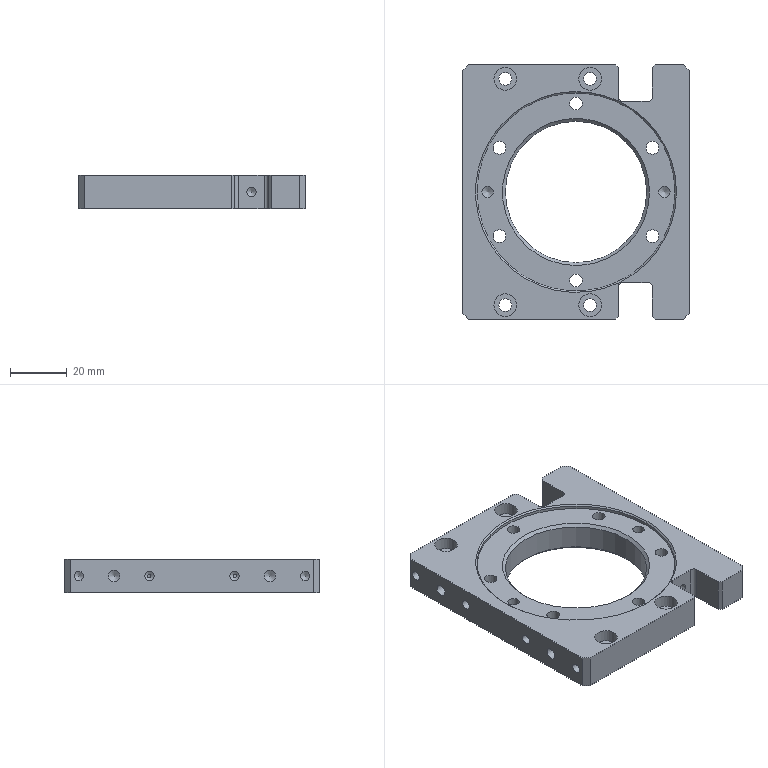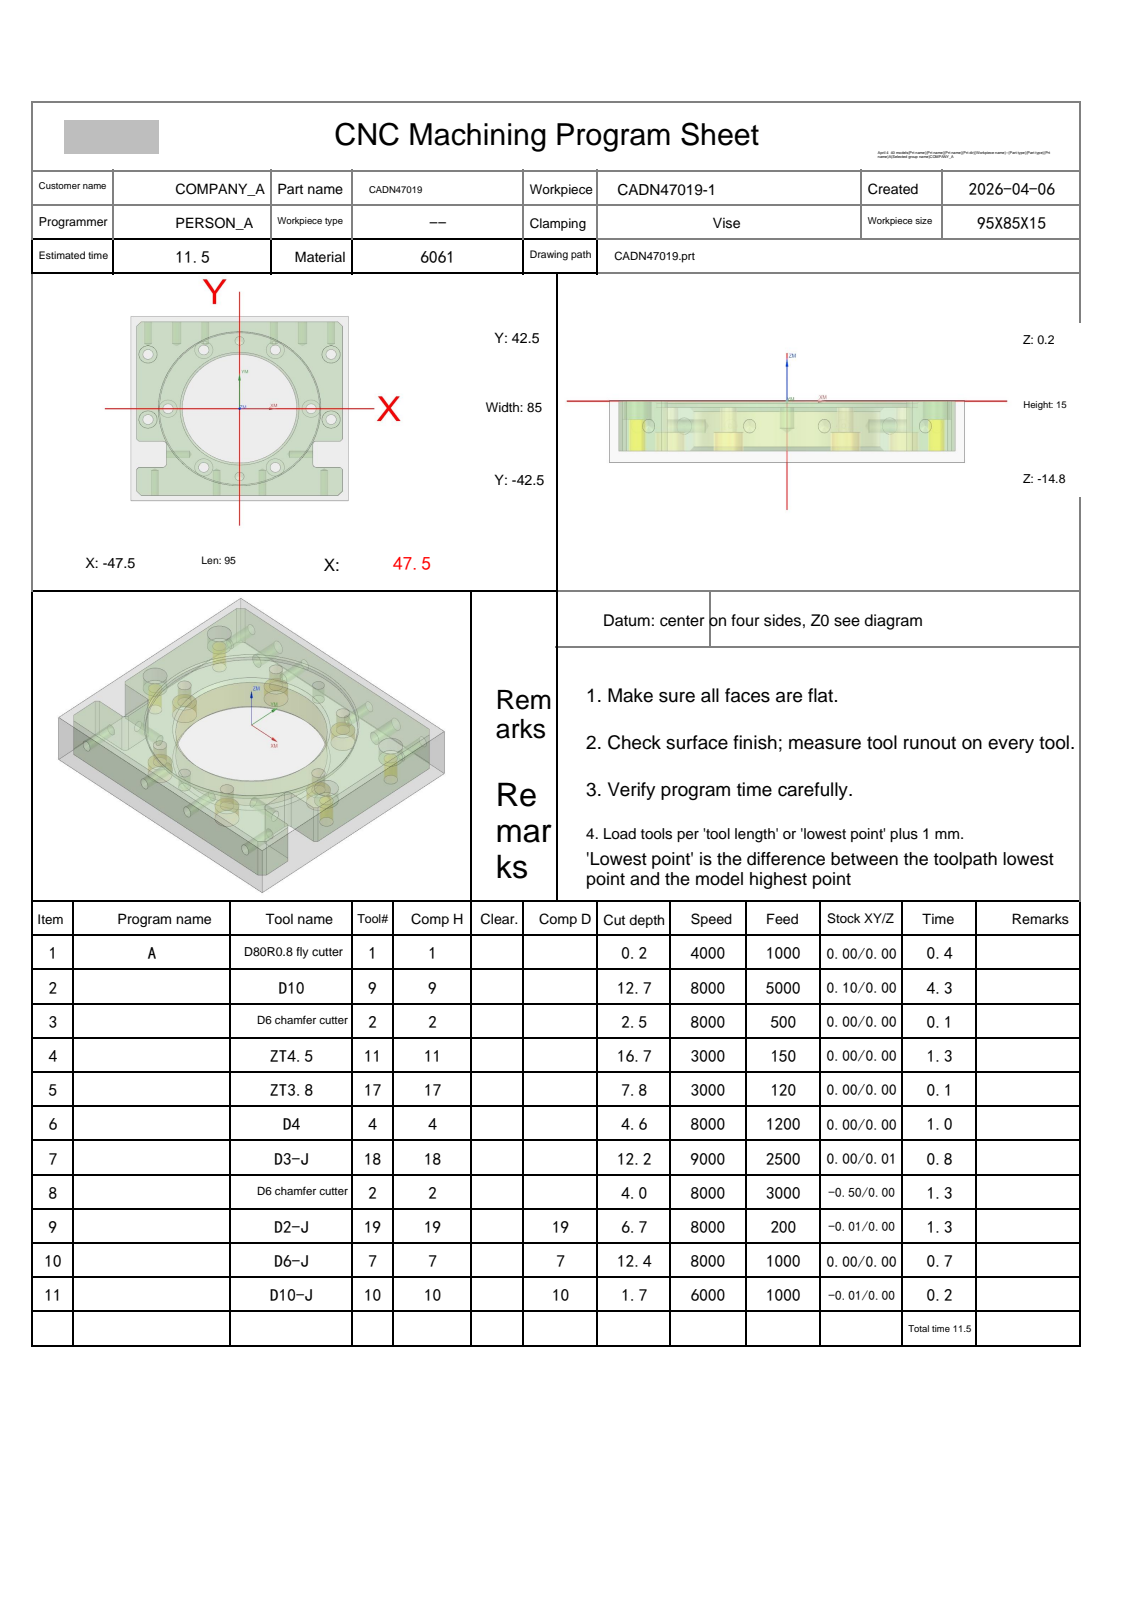NC program | NX | posted by the shop | part box 80 x 90 x 12 mm
Lines 1819 to 2081 of 6628:
N3 T02 M06
(D6 chamfer cutter  D=6. R=0. H=02 ce=0.00 di=0.10)
G00 G90 G54 X0.0 Y0.0 M03 S8000
G43 H02 Z20.
M08
G98 G81 X0.0 Y0.0 Z-.8 R1. F500.
X-15.625 Y-27.063 Z-2.3 R-.5
X0.0 Y-31.25
X15.625 Y-27.063
X31.25 Y0.0
X40. Y-5. Z-.8 R1.
Y25.
X15.625 Y27.063 Z-2.3 R-.5
X0.0 Y31.25
X-15.625 Y27.063
X-40. Y25. Z-.8 R1.
X-31.25 Y0.0 Z-2.3 R-.5
X-40. Y-5. Z-.8 R1.
G80
G00 Z20.
G91 G28 Z0.0
M05
M09
G91 G28 Z0.0
M01
N4 T11 M06
(ZT4.5 D=4.5 DR_a=118 H=11)
G00 G90 G54 X-31.25 Y0.0 M03 S3000
G43 H11 Z20.
M08
G98 G83 X-31.25 Y0.0 Z-16.5 R-.5 F150. Q3.
X-15.625 Y-27.063
X15.625
X31.25 Y0.0
X15.625 Y27.063
X-15.625
G80
G00 Z20.
G00 G90 X40. Y25. M03 S2800
Z20.
G98 G83 X40. Y25. Z-15.352 R1. F100. Q2.
Y-5.
X-40.
Y25.
G80
G00 Z20.
G91 G28 Z0.0
M05
M09
G91 G28 Z0.0
M01
N5 T17 M06
(ZT3.8 D=3.8 DR_a=118 H=17)
G00 G90 G54 X0.0 Y-31.25 M03 S3000
G43 H17 Z20.
M08
G98 G83 X0.0 Y-31.25 Z-7.602 R-.5 F120. Q2.
Y31.25
G80
G00 Z20.
G91 G28 Z0.0
M05
M09
G91 G28 Z0.0
M01
N6 T04 M06
(D4  D=4. R=0. H=04 ce=0.10 di=0.00)
G00 G90 G54 X40. Y25. M03 S8000
G43 H04 Z20.
M08
Z.5
G03 X39.05 Y24.05 I0.0 J-.95 F1200.
X40. Y23.1 I.95 J0.0
X40. Y23.1 Z.2 I0.0 J1.9
X40. Y23.1 Z-.1 I0.0 J1.9
X40. Y23.1 Z-.4 I0.0 J1.9
X40. Y23.1 Z-.7 I0.0 J1.9
X40. Y23.1 Z-1. I0.0 J1.9
X40. Y23.1 Z-1.3 I0.0 J1.9
X40. Y23.1 Z-1.6 I0.0 J1.9
X40. Y23.1 Z-1.9 I0.0 J1.9
X40. Y23.1 Z-2.2 I0.0 J1.9
X40. Y23.1 Z-2.5 I0.0 J1.9
X40. Y23.1 Z-2.8 I0.0 J1.9
X40. Y23.1 Z-3.1 I0.0 J1.9
X40. Y23.1 Z-3.4 I0.0 J1.9
X40. Y23.1 Z-3.7 I0.0 J1.9
X40. Y23.1 Z-4. I0.0 J1.9
X40. Y23.1 Z-4.3 I0.0 J1.9
X41.645 Y25.95 Z-4.4 I0.0 J1.9
X40. Y26.9 I-1.645 J-.95
X38.1 Y25. I0.0 J-1.9
X40. Y23.1 I1.9 J0.0
X41.9 Y25. I0.0 J1.9
X41.645 Y25.95 I-1.9 J0.0
X40.823 Y26.425 I-.823 J-.475
X39.873 Y25.475 I0.0 J-.95
X40. Y25. I.95 J0.0
G00 Z20.
Y-5.
Z.5
G03 X39.05 Y-5.95 I0.0 J-.95
X40. Y-6.9 I.95 J0.0
X40. Y-6.9 Z.2 I0.0 J1.9
X40. Y-6.9 Z-.1 I0.0 J1.9
X40. Y-6.9 Z-.4 I0.0 J1.9
X40. Y-6.9 Z-.7 I0.0 J1.9
X40. Y-6.9 Z-1. I0.0 J1.9
X40. Y-6.9 Z-1.3 I0.0 J1.9
X40. Y-6.9 Z-1.6 I0.0 J1.9
X40. Y-6.9 Z-1.9 I0.0 J1.9
X40. Y-6.9 Z-2.2 I0.0 J1.9
X40. Y-6.9 Z-2.5 I0.0 J1.9
X40. Y-6.9 Z-2.8 I0.0 J1.9
X40. Y-6.9 Z-3.1 I0.0 J1.9
X40. Y-6.9 Z-3.4 I0.0 J1.9
X40. Y-6.9 Z-3.7 I0.0 J1.9
X40. Y-6.9 Z-4. I0.0 J1.9
X40. Y-6.9 Z-4.3 I0.0 J1.9
X41.645 Y-4.05 Z-4.4 I0.0 J1.9
X40. Y-3.1 I-1.645 J-.95
X38.1 Y-5. I0.0 J-1.9
X40. Y-6.9 I1.9 J0.0
X41.9 Y-5. I0.0 J1.9
X41.645 Y-4.05 I-1.9 J0.0
X40.823 Y-3.575 I-.823 J-.475
X39.873 Y-4.525 I0.0 J-.95
X40. Y-5. I.95 J0.0
G00 Z20.
X-40.
Z.5
G03 X-40.95 Y-5.95 I0.0 J-.95
X-40. Y-6.9 I.95 J0.0
X-40. Y-6.9 Z.2 I0.0 J1.9
X-40. Y-6.9 Z-.1 I0.0 J1.9
X-40. Y-6.9 Z-.4 I0.0 J1.9
X-40. Y-6.9 Z-.7 I0.0 J1.9
X-40. Y-6.9 Z-1. I0.0 J1.9
X-40. Y-6.9 Z-1.3 I0.0 J1.9
X-40. Y-6.9 Z-1.6 I0.0 J1.9
X-40. Y-6.9 Z-1.9 I0.0 J1.9
X-40. Y-6.9 Z-2.2 I0.0 J1.9
X-40. Y-6.9 Z-2.5 I0.0 J1.9
X-40. Y-6.9 Z-2.8 I0.0 J1.9
X-40. Y-6.9 Z-3.1 I0.0 J1.9
X-40. Y-6.9 Z-3.4 I0.0 J1.9
X-40. Y-6.9 Z-3.7 I0.0 J1.9
X-40. Y-6.9 Z-4. I0.0 J1.9
X-40. Y-6.9 Z-4.3 I0.0 J1.9
X-38.355 Y-4.05 Z-4.4 I0.0 J1.9
X-40. Y-3.1 I-1.645 J-.95
X-41.9 Y-5. I0.0 J-1.9
X-40. Y-6.9 I1.9 J0.0
X-38.1 Y-5. I0.0 J1.9
X-38.355 Y-4.05 I-1.9 J0.0
X-39.177 Y-3.575 I-.823 J-.475
X-40.127 Y-4.525 I0.0 J-.95
X-40. Y-5. I.95 J0.0
G00 Z20.
Y25.
Z.5
G03 X-40.95 Y24.05 I0.0 J-.95
X-40. Y23.1 I.95 J0.0
X-40. Y23.1 Z.2 I0.0 J1.9
X-40. Y23.1 Z-.1 I0.0 J1.9
X-40. Y23.1 Z-.4 I0.0 J1.9
X-40. Y23.1 Z-.7 I0.0 J1.9
X-40. Y23.1 Z-1. I0.0 J1.9
X-40. Y23.1 Z-1.3 I0.0 J1.9
X-40. Y23.1 Z-1.6 I0.0 J1.9
X-40. Y23.1 Z-1.9 I0.0 J1.9
X-40. Y23.1 Z-2.2 I0.0 J1.9
X-40. Y23.1 Z-2.5 I0.0 J1.9
X-40. Y23.1 Z-2.8 I0.0 J1.9
X-40. Y23.1 Z-3.1 I0.0 J1.9
X-40. Y23.1 Z-3.4 I0.0 J1.9
X-40. Y23.1 Z-3.7 I0.0 J1.9
X-40. Y23.1 Z-4. I0.0 J1.9
X-40. Y23.1 Z-4.3 I0.0 J1.9
X-38.355 Y25.95 Z-4.4 I0.0 J1.9
X-40. Y26.9 I-1.645 J-.95
X-41.9 Y25. I0.0 J-1.9
X-40. Y23.1 I1.9 J0.0
X-38.1 Y25. I0.0 J1.9
X-38.355 Y25.95 I-1.9 J0.0
X-39.177 Y26.425 I-.823 J-.475
X-40.127 Y25.475 I0.0 J-.95
X-40. Y25. I.95 J0.0
G00 Z20.
G00 G90 X40. Y25. M03 S8000
Z20.
Z.5
G41 D04
G01 X39.804 Y24.96 F500.
G03 X39.01 Y23.99 I.196 J-.97
X40. Y23. I.99 J0.0
X39.749 Y23.016 Z-4.4 I0.0 J2.
X40. Y23. I.251 J1.984
X42. Y25. I0.0 J2.
X40. Y27. I-2. J0.0
X38. Y25. I0.0 J-2.
X39.749 Y23.016 I2. J0.0
G01 X39.873 Y23.008
G03 X40.863 Y23.998 I0.0 J.99
X40.19 Y24.936 I-.99 J0.0
G01 G40 X40. Y25.
G00 Z20.
Y-5.
Z.5
G41 D04
G01 X39.804 Y-5.04
G03 X39.01 Y-6.01 I.196 J-.97
X40. Y-7. I.99 J0.0
X39.749 Y-6.984 Z-4.4 I0.0 J2.
X40. Y-7. I.251 J1.984
X42. Y-5. I0.0 J2.
X40. Y-3. I-2. J0.0
X38. Y-5. I0.0 J-2.
X39.749 Y-6.984 I2. J0.0
G01 X39.873 Y-6.992
G03 X40.863 Y-6.002 I0.0 J.99
X40.19 Y-5.064 I-.99 J0.0
G01 G40 X40. Y-5.
G00 Z20.
X-40.
Z.5
G41 D04
G01 X-40.196 Y-5.04
G03 X-40.99 Y-6.01 I.196 J-.97
X-40. Y-7. I.99 J0.0
X-40.251 Y-6.984 Z-4.4 I0.0 J2.
X-40. Y-7. I.251 J1.984
X-38. Y-5. I0.0 J2.
X-40. Y-3. I-2. J0.0
X-42. Y-5. I0.0 J-2.
X-40.251 Y-6.984 I2. J0.0
G01 X-40.127 Y-6.992
G03 X-39.137 Y-6.002 I0.0 J.99
X-39.81 Y-5.064 I-.99 J0.0
G01 G40 X-40. Y-5.
G00 Z20.
Y25.
Z.5
G41 D04
G01 X-40.196 Y24.96
G03 X-40.99 Y23.99 I.196 J-.97
X-40. Y23. I.99 J0.0
X-40.251 Y23.016 Z-4.4 I0.0 J2.
X-40. Y23. I.251 J1.984
X-38. Y25. I0.0 J2.
X-40. Y27. I-2. J0.0
X-42. Y25. I0.0 J-2.
X-40.251 Y23.016 I2. J0.0
G01 X-40.127 Y23.008
G03 X-39.137 Y23.998 I0.0 J.99
X-39.81 Y24.936 I-.99 J0.0
G01 G40 X-40. Y25.
G00 Z20.
G91 G28 Z0.0
M05
M09
G91 G28 Z0.0
M01